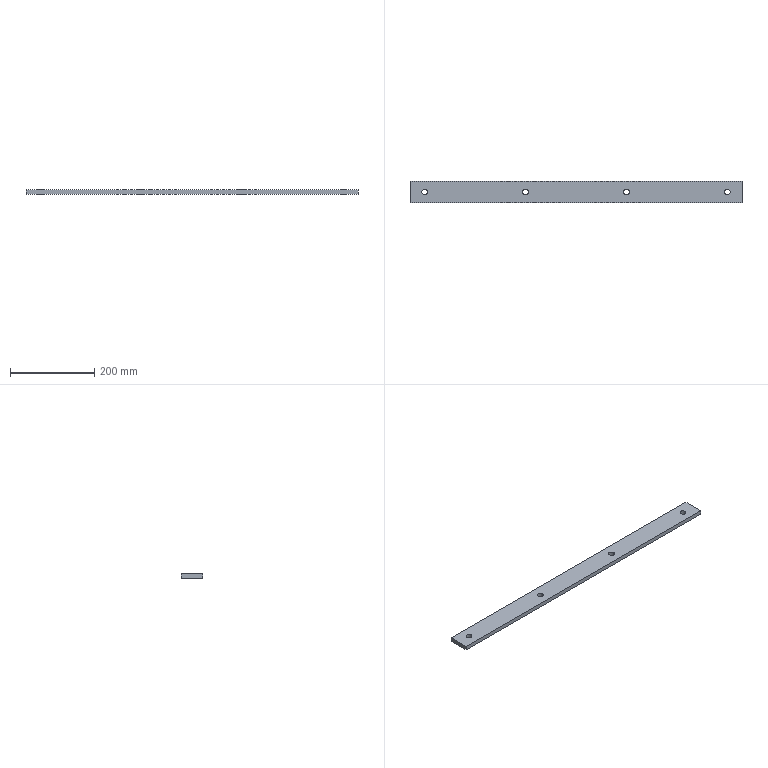Part | NX | features BREP 1 | 1 solid | 14 faces | box 790 x 50 x 10 mm | volume 388842 mm3 | cylinder 8 | plane 6 | commonest cylinder face diameters 14 x8
STEP:
#1=CARTESIAN_POINT('',(113.,0.,-5.));
#2=VERTEX_POINT('',#1);
#3=CARTESIAN_POINT('',(127.,0.,-5.));
#4=VERTEX_POINT('',#3);
#5=CARTESIAN_POINT('',(120.,0.,-5.));
#6=DIRECTION('',(0.,0.,1.));
#7=DIRECTION('',(-1.,0.,0.));
#8=AXIS2_PLACEMENT_3D('',#5,#6,#7);
#9=CIRCLE('',#8,7.);
#10=EDGE_CURVE('',#2,#4,#9,.T.);
#11=ORIENTED_EDGE('',*,*,#10,.F.);
#12=CARTESIAN_POINT('',(113.,0.,5.));
#13=VERTEX_POINT('',#12);
#14=CARTESIAN_POINT('',(113.,0.,-5.));
#15=DIRECTION('',(0.,0.,1.));
#16=VECTOR('',#15,1000.);
#17=LINE('',#14,#16);
#18=EDGE_CURVE('',#2,#13,#17,.T.);
#19=ORIENTED_EDGE('',*,*,#18,.T.);
#20=CARTESIAN_POINT('',(127.,0.,5.));
#21=VERTEX_POINT('',#20);
#22=CARTESIAN_POINT('',(120.,0.,5.));
#23=DIRECTION('',(0.,0.,1.));
#24=DIRECTION('',(-1.,0.,0.));
#25=AXIS2_PLACEMENT_3D('',#22,#23,#24);
#26=CIRCLE('',#25,7.);
#27=EDGE_CURVE('',#13,#21,#26,.T.);
#28=ORIENTED_EDGE('',*,*,#27,.T.);
#29=CARTESIAN_POINT('',(127.,0.,-5.));
#30=DIRECTION('',(0.,0.,1.));
#31=VECTOR('',#30,1000.);
#32=LINE('',#29,#31);
#33=EDGE_CURVE('',#4,#21,#32,.T.);
#34=ORIENTED_EDGE('',*,*,#33,.F.);
#35=EDGE_LOOP('',(#11,#19,#28,#34));
#36=FACE_BOUND('',#35,.T.);
#37=CARTESIAN_POINT('',(120.,0.,-5.));
#38=DIRECTION('',(0.,0.,1.));
#39=DIRECTION('',(-1.,0.,0.));
#40=AXIS2_PLACEMENT_3D('',#37,#38,#39);
#41=CYLINDRICAL_SURFACE('',#40,7.);
#42=ADVANCED_FACE('',(#36),#41,.F.);
#43=CARTESIAN_POINT('',(353.,0.,-5.));
#44=VERTEX_POINT('',#43);
#45=CARTESIAN_POINT('',(367.,0.,-5.));
#46=VERTEX_POINT('',#45);
#47=CARTESIAN_POINT('',(360.,0.,-5.));
#48=DIRECTION('',(0.,0.,1.));
#49=DIRECTION('',(-1.,0.,0.));
#50=AXIS2_PLACEMENT_3D('',#47,#48,#49);
#51=CIRCLE('',#50,7.);
#52=EDGE_CURVE('',#44,#46,#51,.T.);
#53=ORIENTED_EDGE('',*,*,#52,.F.);
#54=CARTESIAN_POINT('',(353.,0.,5.));
#55=VERTEX_POINT('',#54);
#56=CARTESIAN_POINT('',(353.,0.,-5.));
#57=DIRECTION('',(0.,0.,1.));
#58=VECTOR('',#57,1000.);
#59=LINE('',#56,#58);
#60=EDGE_CURVE('',#44,#55,#59,.T.);
#61=ORIENTED_EDGE('',*,*,#60,.T.);
#62=CARTESIAN_POINT('',(367.,0.,5.));
#63=VERTEX_POINT('',#62);
#64=CARTESIAN_POINT('',(360.,0.,5.));
#65=DIRECTION('',(0.,0.,1.));
#66=DIRECTION('',(-1.,0.,0.));
#67=AXIS2_PLACEMENT_3D('',#64,#65,#66);
#68=CIRCLE('',#67,7.);
#69=EDGE_CURVE('',#55,#63,#68,.T.);
#70=ORIENTED_EDGE('',*,*,#69,.T.);
#71=CARTESIAN_POINT('',(367.,0.,-5.));
#72=DIRECTION('',(0.,0.,1.));
#73=VECTOR('',#72,1000.);
#74=LINE('',#71,#73);
#75=EDGE_CURVE('',#46,#63,#74,.T.);
#76=ORIENTED_EDGE('',*,*,#75,.F.);
#77=EDGE_LOOP('',(#53,#61,#70,#76));
#78=FACE_BOUND('',#77,.T.);
#79=CARTESIAN_POINT('',(360.,0.,-5.));
#80=DIRECTION('',(0.,0.,1.));
#81=DIRECTION('',(-1.,0.,0.));
#82=AXIS2_PLACEMENT_3D('',#79,#80,#81);
#83=CYLINDRICAL_SURFACE('',#82,7.);
#84=ADVANCED_FACE('',(#78),#83,.F.);
#85=CARTESIAN_POINT('',(-367.,0.,-5.));
#86=VERTEX_POINT('',#85);
#87=CARTESIAN_POINT('',(-353.,0.,-5.));
#88=VERTEX_POINT('',#87);
#89=CARTESIAN_POINT('',(-360.,0.,-5.));
#90=DIRECTION('',(0.,0.,1.));
#91=DIRECTION('',(1.,0.,0.));
#92=AXIS2_PLACEMENT_3D('',#89,#90,#91);
#93=CIRCLE('',#92,7.);
#94=EDGE_CURVE('',#86,#88,#93,.T.);
#95=ORIENTED_EDGE('',*,*,#94,.F.);
#96=CARTESIAN_POINT('',(-367.,0.,5.));
#97=VERTEX_POINT('',#96);
#98=CARTESIAN_POINT('',(-367.,0.,-5.));
#99=DIRECTION('',(0.,0.,1.));
#100=VECTOR('',#99,1000.);
#101=LINE('',#98,#100);
#102=EDGE_CURVE('',#86,#97,#101,.T.);
#103=ORIENTED_EDGE('',*,*,#102,.T.);
#104=CARTESIAN_POINT('',(-353.,0.,5.));
#105=VERTEX_POINT('',#104);
#106=CARTESIAN_POINT('',(-360.,0.,5.));
#107=DIRECTION('',(0.,0.,1.));
#108=DIRECTION('',(1.,0.,0.));
#109=AXIS2_PLACEMENT_3D('',#106,#107,#108);
#110=CIRCLE('',#109,7.);
#111=EDGE_CURVE('',#97,#105,#110,.T.);
#112=ORIENTED_EDGE('',*,*,#111,.T.);
#113=CARTESIAN_POINT('',(-353.,0.,-5.));
#114=DIRECTION('',(0.,0.,1.));
#115=VECTOR('',#114,1000.);
#116=LINE('',#113,#115);
#117=EDGE_CURVE('',#88,#105,#116,.T.);
#118=ORIENTED_EDGE('',*,*,#117,.F.);
#119=EDGE_LOOP('',(#95,#103,#112,#118));
#120=FACE_BOUND('',#119,.T.);
#121=CARTESIAN_POINT('',(-360.,0.,-5.));
#122=DIRECTION('',(0.,0.,1.));
#123=DIRECTION('',(-1.,0.,0.));
#124=AXIS2_PLACEMENT_3D('',#121,#122,#123);
#125=CYLINDRICAL_SURFACE('',#124,7.);
#126=ADVANCED_FACE('',(#120),#125,.F.);
#127=CARTESIAN_POINT('',(-127.,0.,-5.));
#128=VERTEX_POINT('',#127);
#129=CARTESIAN_POINT('',(-113.,0.,-5.));
#130=VERTEX_POINT('',#129);
#131=CARTESIAN_POINT('',(-120.,0.,-5.));
#132=DIRECTION('',(0.,0.,1.));
#133=DIRECTION('',(1.,0.,0.));
#134=AXIS2_PLACEMENT_3D('',#131,#132,#133);
#135=CIRCLE('',#134,7.);
#136=EDGE_CURVE('',#128,#130,#135,.T.);
#137=ORIENTED_EDGE('',*,*,#136,.F.);
#138=CARTESIAN_POINT('',(-127.,0.,5.));
#139=VERTEX_POINT('',#138);
#140=CARTESIAN_POINT('',(-127.,0.,-5.));
#141=DIRECTION('',(0.,0.,1.));
#142=VECTOR('',#141,1000.);
#143=LINE('',#140,#142);
#144=EDGE_CURVE('',#128,#139,#143,.T.);
#145=ORIENTED_EDGE('',*,*,#144,.T.);
#146=CARTESIAN_POINT('',(-113.,0.,5.));
#147=VERTEX_POINT('',#146);
#148=CARTESIAN_POINT('',(-120.,0.,5.));
#149=DIRECTION('',(0.,0.,1.));
#150=DIRECTION('',(1.,0.,0.));
#151=AXIS2_PLACEMENT_3D('',#148,#149,#150);
#152=CIRCLE('',#151,7.);
#153=EDGE_CURVE('',#139,#147,#152,.T.);
#154=ORIENTED_EDGE('',*,*,#153,.T.);
#155=CARTESIAN_POINT('',(-113.,0.,-5.));
#156=DIRECTION('',(0.,0.,1.));
#157=VECTOR('',#156,1000.);
#158=LINE('',#155,#157);
#159=EDGE_CURVE('',#130,#147,#158,.T.);
#160=ORIENTED_EDGE('',*,*,#159,.F.);
#161=EDGE_LOOP('',(#137,#145,#154,#160));
#162=FACE_BOUND('',#161,.T.);
#163=CARTESIAN_POINT('',(-120.,0.,-5.));
#164=DIRECTION('',(0.,0.,1.));
#165=DIRECTION('',(-1.,0.,0.));
#166=AXIS2_PLACEMENT_3D('',#163,#164,#165);
#167=CYLINDRICAL_SURFACE('',#166,7.);
#168=ADVANCED_FACE('',(#162),#167,.F.);
#169=CARTESIAN_POINT('',(-395.,25.,-5.));
#170=VERTEX_POINT('',#169);
#171=CARTESIAN_POINT('',(-395.,-25.,-5.));
#172=VERTEX_POINT('',#171);
#173=CARTESIAN_POINT('',(-395.,25.,-5.));
#174=DIRECTION('',(0.,-1.,0.));
#175=VECTOR('',#174,1000.);
#176=LINE('',#173,#175);
#177=EDGE_CURVE('',#170,#172,#176,.T.);
#178=ORIENTED_EDGE('',*,*,#177,.T.);
#179=CARTESIAN_POINT('',(-395.,-25.,5.));
#180=VERTEX_POINT('',#179);
#181=CARTESIAN_POINT('',(-395.,-25.,5.));
#182=DIRECTION('',(0.,0.,-1.));
#183=VECTOR('',#182,1000.);
#184=LINE('',#181,#183);
#185=EDGE_CURVE('',#180,#172,#184,.T.);
#186=ORIENTED_EDGE('',*,*,#185,.F.);
#187=CARTESIAN_POINT('',(-395.,25.,5.));
#188=VERTEX_POINT('',#187);
#189=CARTESIAN_POINT('',(-395.,25.,5.));
#190=DIRECTION('',(0.,-1.,0.));
#191=VECTOR('',#190,1000.);
#192=LINE('',#189,#191);
#193=EDGE_CURVE('',#188,#180,#192,.T.);
#194=ORIENTED_EDGE('',*,*,#193,.F.);
#195=CARTESIAN_POINT('',(-395.,25.,5.));
#196=DIRECTION('',(0.,0.,-1.));
#197=VECTOR('',#196,1000.);
#198=LINE('',#195,#197);
#199=EDGE_CURVE('',#188,#170,#198,.T.);
#200=ORIENTED_EDGE('',*,*,#199,.T.);
#201=EDGE_LOOP('',(#178,#186,#194,#200));
#202=FACE_BOUND('',#201,.T.);
#203=CARTESIAN_POINT('',(-395.,25.,5.));
#204=DIRECTION('',(1.,0.,0.));
#205=DIRECTION('',(0.,0.,1.));
#206=AXIS2_PLACEMENT_3D('',#203,#204,#205);
#207=PLANE('',#206);
#208=ADVANCED_FACE('',(#202),#207,.F.);
#209=CARTESIAN_POINT('',(395.,-25.,-5.));
#210=VERTEX_POINT('',#209);
#211=CARTESIAN_POINT('',(-395.,-25.,-5.));
#212=DIRECTION('',(1.,0.,0.));
#213=VECTOR('',#212,1000.);
#214=LINE('',#211,#213);
#215=EDGE_CURVE('',#172,#210,#214,.T.);
#216=ORIENTED_EDGE('',*,*,#215,.T.);
#217=CARTESIAN_POINT('',(395.,-25.,5.));
#218=VERTEX_POINT('',#217);
#219=CARTESIAN_POINT('',(395.,-25.,5.));
#220=DIRECTION('',(0.,0.,-1.));
#221=VECTOR('',#220,1000.);
#222=LINE('',#219,#221);
#223=EDGE_CURVE('',#218,#210,#222,.T.);
#224=ORIENTED_EDGE('',*,*,#223,.F.);
#225=CARTESIAN_POINT('',(-395.,-25.,5.));
#226=DIRECTION('',(1.,0.,0.));
#227=VECTOR('',#226,1000.);
#228=LINE('',#225,#227);
#229=EDGE_CURVE('',#180,#218,#228,.T.);
#230=ORIENTED_EDGE('',*,*,#229,.F.);
#231=ORIENTED_EDGE('',*,*,#185,.T.);
#232=EDGE_LOOP('',(#216,#224,#230,#231));
#233=FACE_BOUND('',#232,.T.);
#234=CARTESIAN_POINT('',(-395.,-25.,5.));
#235=DIRECTION('',(0.,1.,0.));
#236=DIRECTION('',(0.,0.,-1.));
#237=AXIS2_PLACEMENT_3D('',#234,#235,#236);
#238=PLANE('',#237);
#239=ADVANCED_FACE('',(#233),#238,.F.);
#240=CARTESIAN_POINT('',(395.,25.,-5.));
#241=VERTEX_POINT('',#240);
#242=CARTESIAN_POINT('',(395.,25.,-5.));
#243=DIRECTION('',(0.,1.,0.));
#244=VECTOR('',#243,1000.);
#245=LINE('',#242,#244);
#246=EDGE_CURVE('',#210,#241,#245,.T.);
#247=ORIENTED_EDGE('',*,*,#246,.T.);
#248=CARTESIAN_POINT('',(395.,25.,5.));
#249=VERTEX_POINT('',#248);
#250=CARTESIAN_POINT('',(395.,25.,5.));
#251=DIRECTION('',(0.,0.,-1.));
#252=VECTOR('',#251,1000.);
#253=LINE('',#250,#252);
#254=EDGE_CURVE('',#249,#241,#253,.T.);
#255=ORIENTED_EDGE('',*,*,#254,.F.);
#256=CARTESIAN_POINT('',(395.,25.,5.));
#257=DIRECTION('',(0.,1.,0.));
#258=VECTOR('',#257,1000.);
#259=LINE('',#256,#258);
#260=EDGE_CURVE('',#218,#249,#259,.T.);
#261=ORIENTED_EDGE('',*,*,#260,.F.);
#262=ORIENTED_EDGE('',*,*,#223,.T.);
#263=EDGE_LOOP('',(#247,#255,#261,#262));
#264=FACE_BOUND('',#263,.T.);
#265=CARTESIAN_POINT('',(395.,25.,5.));
#266=DIRECTION('',(-1.,0.,0.));
#267=DIRECTION('',(0.,0.,-1.));
#268=AXIS2_PLACEMENT_3D('',#265,#266,#267);
#269=PLANE('',#268);
#270=ADVANCED_FACE('',(#264),#269,.F.);
#271=CARTESIAN_POINT('',(-395.,25.,-5.));
#272=DIRECTION('',(-1.,0.,0.));
#273=VECTOR('',#272,1000.);
#274=LINE('',#271,#273);
#275=EDGE_CURVE('',#241,#170,#274,.T.);
#276=ORIENTED_EDGE('',*,*,#275,.T.);
#277=ORIENTED_EDGE('',*,*,#199,.F.);
#278=CARTESIAN_POINT('',(-395.,25.,5.));
#279=DIRECTION('',(-1.,0.,0.));
#280=VECTOR('',#279,1000.);
#281=LINE('',#278,#280);
#282=EDGE_CURVE('',#249,#188,#281,.T.);
#283=ORIENTED_EDGE('',*,*,#282,.F.);
#284=ORIENTED_EDGE('',*,*,#254,.T.);
#285=EDGE_LOOP('',(#276,#277,#283,#284));
#286=FACE_BOUND('',#285,.T.);
#287=CARTESIAN_POINT('',(-395.,25.,5.));
#288=DIRECTION('',(0.,-1.,0.));
#289=DIRECTION('',(0.,0.,1.));
#290=AXIS2_PLACEMENT_3D('',#287,#288,#289);
#291=PLANE('',#290);
#292=ADVANCED_FACE('',(#286),#291,.F.);
#293=CARTESIAN_POINT('',(120.,0.,5.));
#294=DIRECTION('',(0.,0.,1.));
#295=DIRECTION('',(-1.,0.,0.));
#296=AXIS2_PLACEMENT_3D('',#293,#294,#295);
#297=CIRCLE('',#296,7.);
#298=EDGE_CURVE('',#21,#13,#297,.T.);
#299=ORIENTED_EDGE('',*,*,#298,.F.);
#300=ORIENTED_EDGE('',*,*,#27,.F.);
#301=EDGE_LOOP('',(#299,#300));
#302=FACE_BOUND('',#301,.T.);
#303=CARTESIAN_POINT('',(360.,0.,5.));
#304=DIRECTION('',(0.,0.,1.));
#305=DIRECTION('',(-1.,0.,0.));
#306=AXIS2_PLACEMENT_3D('',#303,#304,#305);
#307=CIRCLE('',#306,7.);
#308=EDGE_CURVE('',#63,#55,#307,.T.);
#309=ORIENTED_EDGE('',*,*,#308,.F.);
#310=ORIENTED_EDGE('',*,*,#69,.F.);
#311=EDGE_LOOP('',(#309,#310));
#312=FACE_BOUND('',#311,.T.);
#313=CARTESIAN_POINT('',(-360.,0.,5.));
#314=DIRECTION('',(0.,0.,1.));
#315=DIRECTION('',(1.,0.,0.));
#316=AXIS2_PLACEMENT_3D('',#313,#314,#315);
#317=CIRCLE('',#316,7.);
#318=EDGE_CURVE('',#105,#97,#317,.T.);
#319=ORIENTED_EDGE('',*,*,#318,.F.);
#320=ORIENTED_EDGE('',*,*,#111,.F.);
#321=EDGE_LOOP('',(#319,#320));
#322=FACE_BOUND('',#321,.T.);
#323=CARTESIAN_POINT('',(-120.,0.,5.));
#324=DIRECTION('',(0.,0.,1.));
#325=DIRECTION('',(1.,0.,0.));
#326=AXIS2_PLACEMENT_3D('',#323,#324,#325);
#327=CIRCLE('',#326,7.);
#328=EDGE_CURVE('',#147,#139,#327,.T.);
#329=ORIENTED_EDGE('',*,*,#328,.F.);
#330=ORIENTED_EDGE('',*,*,#153,.F.);
#331=EDGE_LOOP('',(#329,#330));
#332=FACE_BOUND('',#331,.T.);
#333=ORIENTED_EDGE('',*,*,#193,.T.);
#334=ORIENTED_EDGE('',*,*,#229,.T.);
#335=ORIENTED_EDGE('',*,*,#260,.T.);
#336=ORIENTED_EDGE('',*,*,#282,.T.);
#337=EDGE_LOOP('',(#333,#334,#335,#336));
#338=FACE_BOUND('',#337,.T.);
#339=CARTESIAN_POINT('',(-395.,-25.,5.));
#340=DIRECTION('',(0.,0.,1.));
#341=DIRECTION('',(-1.,0.,0.));
#342=AXIS2_PLACEMENT_3D('',#339,#340,#341);
#343=PLANE('',#342);
#344=ADVANCED_FACE('',(#302,#312,#322,#332,#338),#343,.T.);
#345=CARTESIAN_POINT('',(120.,0.,-5.));
#346=DIRECTION('',(0.,0.,1.));
#347=DIRECTION('',(-1.,0.,0.));
#348=AXIS2_PLACEMENT_3D('',#345,#346,#347);
#349=CIRCLE('',#348,7.);
#350=EDGE_CURVE('',#4,#2,#349,.T.);
#351=ORIENTED_EDGE('',*,*,#350,.T.);
#352=ORIENTED_EDGE('',*,*,#10,.T.);
#353=EDGE_LOOP('',(#351,#352));
#354=FACE_BOUND('',#353,.T.);
#355=CARTESIAN_POINT('',(360.,0.,-5.));
#356=DIRECTION('',(0.,0.,1.));
#357=DIRECTION('',(-1.,0.,0.));
#358=AXIS2_PLACEMENT_3D('',#355,#356,#357);
#359=CIRCLE('',#358,7.);
#360=EDGE_CURVE('',#46,#44,#359,.T.);
#361=ORIENTED_EDGE('',*,*,#360,.T.);
#362=ORIENTED_EDGE('',*,*,#52,.T.);
#363=EDGE_LOOP('',(#361,#362));
#364=FACE_BOUND('',#363,.T.);
#365=CARTESIAN_POINT('',(-360.,0.,-5.));
#366=DIRECTION('',(0.,0.,1.));
#367=DIRECTION('',(1.,0.,0.));
#368=AXIS2_PLACEMENT_3D('',#365,#366,#367);
#369=CIRCLE('',#368,7.);
#370=EDGE_CURVE('',#88,#86,#369,.T.);
#371=ORIENTED_EDGE('',*,*,#370,.T.);
#372=ORIENTED_EDGE('',*,*,#94,.T.);
#373=EDGE_LOOP('',(#371,#372));
#374=FACE_BOUND('',#373,.T.);
#375=CARTESIAN_POINT('',(-120.,0.,-5.));
#376=DIRECTION('',(0.,0.,1.));
#377=DIRECTION('',(1.,0.,0.));
#378=AXIS2_PLACEMENT_3D('',#375,#376,#377);
#379=CIRCLE('',#378,7.);
#380=EDGE_CURVE('',#130,#128,#379,.T.);
#381=ORIENTED_EDGE('',*,*,#380,.T.);
#382=ORIENTED_EDGE('',*,*,#136,.T.);
#383=EDGE_LOOP('',(#381,#382));
#384=FACE_BOUND('',#383,.T.);
#385=ORIENTED_EDGE('',*,*,#177,.F.);
#386=ORIENTED_EDGE('',*,*,#275,.F.);
#387=ORIENTED_EDGE('',*,*,#246,.F.);
#388=ORIENTED_EDGE('',*,*,#215,.F.);
#389=EDGE_LOOP('',(#385,#386,#387,#388));
#390=FACE_BOUND('',#389,.T.);
#391=CARTESIAN_POINT('',(-395.,-25.,-5.));
#392=DIRECTION('',(0.,0.,1.));
#393=DIRECTION('',(-1.,0.,0.));
#394=AXIS2_PLACEMENT_3D('',#391,#392,#393);
#395=PLANE('',#394);
#396=ADVANCED_FACE('',(#354,#364,#374,#384,#390),#395,.F.);
#397=ORIENTED_EDGE('',*,*,#144,.F.);
#398=ORIENTED_EDGE('',*,*,#380,.F.);
#399=ORIENTED_EDGE('',*,*,#159,.T.);
#400=ORIENTED_EDGE('',*,*,#328,.T.);
#401=EDGE_LOOP('',(#397,#398,#399,#400));
#402=FACE_BOUND('',#401,.T.);
#403=CARTESIAN_POINT('',(-120.,0.,-5.));
#404=DIRECTION('',(0.,0.,1.));
#405=DIRECTION('',(-1.,0.,0.));
#406=AXIS2_PLACEMENT_3D('',#403,#404,#405);
#407=CYLINDRICAL_SURFACE('',#406,7.);
#408=ADVANCED_FACE('',(#402),#407,.F.);
#409=ORIENTED_EDGE('',*,*,#102,.F.);
#410=ORIENTED_EDGE('',*,*,#370,.F.);
#411=ORIENTED_EDGE('',*,*,#117,.T.);
#412=ORIENTED_EDGE('',*,*,#318,.T.);
#413=EDGE_LOOP('',(#409,#410,#411,#412));
#414=FACE_BOUND('',#413,.T.);
#415=CARTESIAN_POINT('',(-360.,0.,-5.));
#416=DIRECTION('',(0.,0.,1.));
#417=DIRECTION('',(-1.,0.,0.));
#418=AXIS2_PLACEMENT_3D('',#415,#416,#417);
#419=CYLINDRICAL_SURFACE('',#418,7.);
#420=ADVANCED_FACE('',(#414),#419,.F.);
#421=ORIENTED_EDGE('',*,*,#60,.F.);
#422=ORIENTED_EDGE('',*,*,#360,.F.);
#423=ORIENTED_EDGE('',*,*,#75,.T.);
#424=ORIENTED_EDGE('',*,*,#308,.T.);
#425=EDGE_LOOP('',(#421,#422,#423,#424));
#426=FACE_BOUND('',#425,.T.);
#427=CARTESIAN_POINT('',(360.,0.,-5.));
#428=DIRECTION('',(0.,0.,1.));
#429=DIRECTION('',(-1.,0.,0.));
#430=AXIS2_PLACEMENT_3D('',#427,#428,#429);
#431=CYLINDRICAL_SURFACE('',#430,7.);
#432=ADVANCED_FACE('',(#426),#431,.F.);
#433=ORIENTED_EDGE('',*,*,#18,.F.);
#434=ORIENTED_EDGE('',*,*,#350,.F.);
#435=ORIENTED_EDGE('',*,*,#33,.T.);
#436=ORIENTED_EDGE('',*,*,#298,.T.);
#437=EDGE_LOOP('',(#433,#434,#435,#436));
#438=FACE_BOUND('',#437,.T.);
#439=CARTESIAN_POINT('',(120.,0.,-5.));
#440=DIRECTION('',(0.,0.,1.));
#441=DIRECTION('',(-1.,0.,0.));
#442=AXIS2_PLACEMENT_3D('',#439,#440,#441);
#443=CYLINDRICAL_SURFACE('',#442,7.);
#444=ADVANCED_FACE('',(#438),#443,.F.);
#445=CLOSED_SHELL('',(#42,#84,#126,#168,#208,#239,#270,#292,#344,#396,#408,#420,#432,#444));
#446=MANIFOLD_SOLID_BREP('',#445);
#447=(LENGTH_UNIT()NAMED_UNIT(*)SI_UNIT(.MILLI.,.METRE.));
#448=UNCERTAINTY_MEASURE_WITH_UNIT(LENGTH_MEASURE(0.00001),#447,'','');
#449=(NAMED_UNIT(*)PLANE_ANGLE_UNIT()SI_UNIT($,.RADIAN.));
#450=(NAMED_UNIT(*)SI_UNIT($,.STERADIAN.)SOLID_ANGLE_UNIT());
#451=(GEOMETRIC_REPRESENTATION_CONTEXT(3)GLOBAL_UNCERTAINTY_ASSIGNED_CONTEXT((#448))GLOBAL_UNIT_ASSIGNED_CONTEXT((#447,#449,#450))REPRESENTATION_CONTEXT('',''));
#452=ADVANCED_BREP_SHAPE_REPRESENTATION('',(#446),#451);